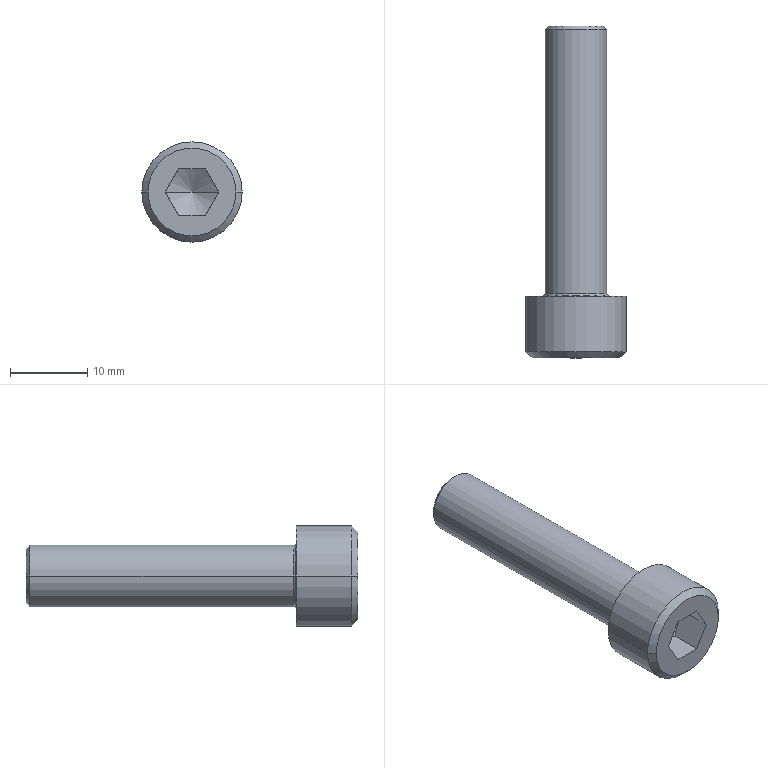Part | Creo | 1 solid | 23 faces | box 13 x 43 x 13 mm | volume 2657 mm3 | plane 9 | cone 6 | cylinder 4 | torus 4 | commonest cylinder face diameters 8 x2 13 x2
STEP:
#1=CARTESIAN_POINT('',(0.,0.,0.));
#2=DIRECTION('',(0.,0.,1.));
#3=DIRECTION('',(1.,0.,0.));
#4=AXIS2_PLACEMENT_3D('',#1,#2,#3);
#5=CARTESIAN_POINT('',(73.036,-244.,-213.));
#6=VERTEX_POINT('',#5);
#7=CARTESIAN_POINT('',(74.768,-244.,-216.));
#8=VERTEX_POINT('',#7);
#9=CARTESIAN_POINT('',(73.036,-244.,-213.));
#10=CARTESIAN_POINT('',(73.087,-243.971,-213.088));
#11=CARTESIAN_POINT('',(73.187,-243.917,-213.261));
#12=CARTESIAN_POINT('',(73.331,-243.851,-213.511));
#13=CARTESIAN_POINT('',(73.473,-243.799,-213.757));
#14=CARTESIAN_POINT('',(73.614,-243.761,-214.002));
#15=CARTESIAN_POINT('',(73.758,-243.737,-214.25));
#16=CARTESIAN_POINT('',(73.902,-243.729,-214.5));
#17=CARTESIAN_POINT('',(74.046,-243.737,-214.75));
#18=CARTESIAN_POINT('',(74.19,-243.761,-214.998));
#19=CARTESIAN_POINT('',(74.331,-243.799,-215.243));
#20=CARTESIAN_POINT('',(74.473,-243.851,-215.489));
#21=CARTESIAN_POINT('',(74.617,-243.917,-215.739));
#22=CARTESIAN_POINT('',(74.717,-243.971,-215.912));
#23=CARTESIAN_POINT('',(74.768,-244.,-216.));
#24=B_SPLINE_CURVE_WITH_KNOTS('',3,(#9,#10,#11,#12,#13,#14,#15,#16,#17,#18,#19,#20,#21,#22,#23),.UNSPECIFIED.,.F.,.F.,(4,1,1,1,1,1,1,1,1,1,1,1,4),(0.,0.08333,0.1667,0.25,0.3333,0.4167,0.5,0.5833,0.6667,0.75,0.8333,0.9167,1.),.UNSPECIFIED.);
#25=EDGE_CURVE('',#6,#8,#24,.T.);
#26=ORIENTED_EDGE('',*,*,#25,.F.);
#27=CARTESIAN_POINT('',(76.5,-242.,-213.));
#28=VERTEX_POINT('',#27);
#29=CARTESIAN_POINT('',(76.5,-242.,-213.));
#30=DIRECTION('',(-0.866,-0.5,0.));
#31=VECTOR('',#30,4.);
#32=LINE('',#29,#31);
#33=EDGE_CURVE('',#28,#6,#32,.T.);
#34=ORIENTED_EDGE('',*,*,#33,.F.);
#35=CARTESIAN_POINT('',(79.964,-244.,-213.));
#36=VERTEX_POINT('',#35);
#37=CARTESIAN_POINT('',(76.5,-242.,-213.));
#38=DIRECTION('',(0.866,-0.5,0.));
#39=VECTOR('',#38,4.);
#40=LINE('',#37,#39);
#41=EDGE_CURVE('',#28,#36,#40,.T.);
#42=ORIENTED_EDGE('',*,*,#41,.T.);
#43=CARTESIAN_POINT('',(78.232,-244.,-216.));
#44=VERTEX_POINT('',#43);
#45=CARTESIAN_POINT('',(78.232,-244.,-216.));
#46=CARTESIAN_POINT('',(78.283,-243.971,-215.912));
#47=CARTESIAN_POINT('',(78.383,-243.917,-215.739));
#48=CARTESIAN_POINT('',(78.527,-243.851,-215.489));
#49=CARTESIAN_POINT('',(78.669,-243.799,-215.243));
#50=CARTESIAN_POINT('',(78.81,-243.761,-214.998));
#51=CARTESIAN_POINT('',(78.954,-243.737,-214.75));
#52=CARTESIAN_POINT('',(79.098,-243.729,-214.5));
#53=CARTESIAN_POINT('',(79.242,-243.737,-214.25));
#54=CARTESIAN_POINT('',(79.386,-243.761,-214.002));
#55=CARTESIAN_POINT('',(79.527,-243.799,-213.757));
#56=CARTESIAN_POINT('',(79.669,-243.851,-213.511));
#57=CARTESIAN_POINT('',(79.813,-243.917,-213.261));
#58=CARTESIAN_POINT('',(79.913,-243.971,-213.088));
#59=CARTESIAN_POINT('',(79.964,-244.,-213.));
#60=B_SPLINE_CURVE_WITH_KNOTS('',3,(#45,#46,#47,#48,#49,#50,#51,#52,#53,#54,#55,#56,#57,#58,#59),.UNSPECIFIED.,.F.,.F.,(4,1,1,1,1,1,1,1,1,1,1,1,4),(0.,0.08333,0.1667,0.25,0.3333,0.4167,0.5,0.5833,0.6667,0.75,0.8333,0.9167,1.),.UNSPECIFIED.);
#61=EDGE_CURVE('',#44,#36,#60,.T.);
#62=ORIENTED_EDGE('',*,*,#61,.F.);
#63=CARTESIAN_POINT('',(74.768,-244.,-216.));
#64=CARTESIAN_POINT('',(74.869,-243.971,-216.));
#65=CARTESIAN_POINT('',(75.069,-243.917,-216.));
#66=CARTESIAN_POINT('',(75.357,-243.851,-216.));
#67=CARTESIAN_POINT('',(75.641,-243.799,-216.));
#68=CARTESIAN_POINT('',(75.924,-243.761,-216.));
#69=CARTESIAN_POINT('',(76.211,-243.737,-216.));
#70=CARTESIAN_POINT('',(76.5,-243.729,-216.));
#71=CARTESIAN_POINT('',(76.789,-243.737,-216.));
#72=CARTESIAN_POINT('',(77.076,-243.761,-216.));
#73=CARTESIAN_POINT('',(77.359,-243.799,-216.));
#74=CARTESIAN_POINT('',(77.643,-243.851,-216.));
#75=CARTESIAN_POINT('',(77.931,-243.917,-216.));
#76=CARTESIAN_POINT('',(78.131,-243.971,-216.));
#77=CARTESIAN_POINT('',(78.232,-244.,-216.));
#78=B_SPLINE_CURVE_WITH_KNOTS('',3,(#63,#64,#65,#66,#67,#68,#69,#70,#71,#72,#73,#74,#75,#76,#77),.UNSPECIFIED.,.F.,.F.,(4,1,1,1,1,1,1,1,1,1,1,1,4),(0.,0.08333,0.1667,0.25,0.3333,0.4167,0.5,0.5833,0.6667,0.75,0.8333,0.9167,1.),.UNSPECIFIED.);
#79=EDGE_CURVE('',#8,#44,#78,.T.);
#80=ORIENTED_EDGE('',*,*,#79,.F.);
#81=EDGE_LOOP('',(#26,#34,#42,#62,#80));
#82=FACE_OUTER_BOUND('',#81,.F.);
#83=CARTESIAN_POINT('',(76.5,-243.02,-213.));
#84=DIRECTION('',(0.,-1.,0.));
#85=DIRECTION('',(-1.,0.,0.));
#86=AXIS2_PLACEMENT_3D('',#83,#84,#85);
#87=CONICAL_SURFACE('',#86,1.767,60.);
#88=ADVANCED_FACE('',(#82),#87,.F.);
#89=CARTESIAN_POINT('',(74.768,-248.,-216.));
#90=VERTEX_POINT('',#89);
#91=CARTESIAN_POINT('',(73.036,-248.,-213.));
#92=VERTEX_POINT('',#91);
#93=CARTESIAN_POINT('',(74.768,-248.,-216.));
#94=DIRECTION('',(-0.5,0.,0.866));
#95=VECTOR('',#94,3.464);
#96=LINE('',#93,#95);
#97=EDGE_CURVE('',#90,#92,#96,.T.);
#98=ORIENTED_EDGE('',*,*,#97,.T.);
#99=CARTESIAN_POINT('',(73.036,-248.,-213.));
#100=DIRECTION('',(0.,1.,0.));
#101=VECTOR('',#100,4.);
#102=LINE('',#99,#101);
#103=EDGE_CURVE('',#92,#6,#102,.T.);
#104=ORIENTED_EDGE('',*,*,#103,.T.);
#105=ORIENTED_EDGE('',*,*,#25,.T.);
#106=CARTESIAN_POINT('',(74.768,-248.,-216.));
#107=DIRECTION('',(0.,1.,0.));
#108=VECTOR('',#107,4.);
#109=LINE('',#106,#108);
#110=EDGE_CURVE('',#90,#8,#109,.T.);
#111=ORIENTED_EDGE('',*,*,#110,.F.);
#112=EDGE_LOOP('',(#98,#104,#105,#111));
#113=FACE_OUTER_BOUND('',#112,.F.);
#114=CARTESIAN_POINT('',(74.768,-244.,-216.));
#115=DIRECTION('',(0.866,0.,0.5));
#116=DIRECTION('',(-0.5,0.,0.866));
#117=AXIS2_PLACEMENT_3D('',#114,#115,#116);
#118=PLANE('',#117);
#119=ADVANCED_FACE('',(#113),#118,.T.);
#120=CARTESIAN_POINT('',(70.8,-248.,-213.));
#121=VERTEX_POINT('',#120);
#122=CARTESIAN_POINT('',(82.2,-248.,-213.));
#123=VERTEX_POINT('',#122);
#124=CARTESIAN_POINT('',(76.5,-248.,-213.));
#125=DIRECTION('',(0.,-1.,0.));
#126=DIRECTION('',(-1.,0.,0.));
#127=AXIS2_PLACEMENT_3D('',#124,#125,#126);
#128=CIRCLE('',#127,5.7);
#129=EDGE_CURVE('',#121,#123,#128,.T.);
#130=ORIENTED_EDGE('',*,*,#129,.F.);
#131=CARTESIAN_POINT('',(76.5,-248.,-213.));
#132=DIRECTION('',(0.,-1.,0.));
#133=DIRECTION('',(1.,0.,0.));
#134=AXIS2_PLACEMENT_3D('',#131,#132,#133);
#135=CIRCLE('',#134,5.7);
#136=EDGE_CURVE('',#123,#121,#135,.T.);
#137=ORIENTED_EDGE('',*,*,#136,.F.);
#138=EDGE_LOOP('',(#130,#137));
#139=FACE_OUTER_BOUND('',#138,.F.);
#140=CARTESIAN_POINT('',(74.768,-248.,-210.));
#141=VERTEX_POINT('',#140);
#142=CARTESIAN_POINT('',(73.036,-248.,-213.));
#143=DIRECTION('',(0.5,0.,0.866));
#144=VECTOR('',#143,3.464);
#145=LINE('',#142,#144);
#146=EDGE_CURVE('',#92,#141,#145,.T.);
#147=ORIENTED_EDGE('',*,*,#146,.F.);
#148=ORIENTED_EDGE('',*,*,#97,.F.);
#149=CARTESIAN_POINT('',(78.232,-248.,-216.));
#150=VERTEX_POINT('',#149);
#151=CARTESIAN_POINT('',(74.768,-248.,-216.));
#152=DIRECTION('',(1.,0.,0.));
#153=VECTOR('',#152,3.464);
#154=LINE('',#151,#153);
#155=EDGE_CURVE('',#90,#150,#154,.T.);
#156=ORIENTED_EDGE('',*,*,#155,.T.);
#157=CARTESIAN_POINT('',(79.964,-248.,-213.));
#158=VERTEX_POINT('',#157);
#159=CARTESIAN_POINT('',(79.964,-248.,-213.));
#160=DIRECTION('',(-0.5,0.,-0.866));
#161=VECTOR('',#160,3.464);
#162=LINE('',#159,#161);
#163=EDGE_CURVE('',#158,#150,#162,.T.);
#164=ORIENTED_EDGE('',*,*,#163,.F.);
#165=CARTESIAN_POINT('',(78.232,-248.,-210.));
#166=VERTEX_POINT('',#165);
#167=CARTESIAN_POINT('',(78.232,-248.,-210.));
#168=DIRECTION('',(0.5,0.,-0.866));
#169=VECTOR('',#168,3.464);
#170=LINE('',#167,#169);
#171=EDGE_CURVE('',#166,#158,#170,.T.);
#172=ORIENTED_EDGE('',*,*,#171,.F.);
#173=CARTESIAN_POINT('',(78.232,-248.,-210.));
#174=DIRECTION('',(-1.,0.,0.));
#175=VECTOR('',#174,3.464);
#176=LINE('',#173,#175);
#177=EDGE_CURVE('',#166,#141,#176,.T.);
#178=ORIENTED_EDGE('',*,*,#177,.T.);
#179=EDGE_LOOP('',(#147,#148,#156,#164,#172,#178));
#180=FACE_BOUND('',#179,.F.);
#181=CARTESIAN_POINT('',(76.5,-248.,-213.));
#182=DIRECTION('',(0.,-1.,0.));
#183=DIRECTION('',(-1.,0.,0.));
#184=AXIS2_PLACEMENT_3D('',#181,#182,#183);
#185=PLANE('',#184);
#186=ADVANCED_FACE('',(#139,#180),#185,.T.);
#187=CARTESIAN_POINT('',(70.,-247.2,-213.));
#188=VERTEX_POINT('',#187);
#189=CARTESIAN_POINT('',(83.,-247.2,-213.));
#190=VERTEX_POINT('',#189);
#191=CARTESIAN_POINT('',(76.5,-247.2,-213.));
#192=DIRECTION('',(0.,-1.,0.));
#193=DIRECTION('',(-1.,0.,0.));
#194=AXIS2_PLACEMENT_3D('',#191,#192,#193);
#195=CIRCLE('',#194,6.5);
#196=EDGE_CURVE('',#188,#190,#195,.T.);
#197=ORIENTED_EDGE('',*,*,#196,.F.);
#198=CARTESIAN_POINT('',(70.8,-248.,-213.));
#199=DIRECTION('',(-0.7071,0.7071,0.));
#200=VECTOR('',#199,1.131);
#201=LINE('',#198,#200);
#202=EDGE_CURVE('',#121,#188,#201,.T.);
#203=ORIENTED_EDGE('',*,*,#202,.F.);
#204=ORIENTED_EDGE('',*,*,#129,.T.);
#205=CARTESIAN_POINT('',(82.2,-248.,-213.));
#206=DIRECTION('',(0.7071,0.7071,0.));
#207=VECTOR('',#206,1.131);
#208=LINE('',#205,#207);
#209=EDGE_CURVE('',#123,#190,#208,.T.);
#210=ORIENTED_EDGE('',*,*,#209,.T.);
#211=EDGE_LOOP('',(#197,#203,#204,#210));
#212=FACE_OUTER_BOUND('',#211,.F.);
#213=CARTESIAN_POINT('',(76.5,-247.6,-213.));
#214=DIRECTION('',(0.,1.,0.));
#215=DIRECTION('',(1.,0.,0.));
#216=AXIS2_PLACEMENT_3D('',#213,#214,#215);
#217=CONICAL_SURFACE('',#216,6.1,45.);
#218=ADVANCED_FACE('',(#212),#217,.T.);
#219=ORIENTED_EDGE('',*,*,#196,.T.);
#220=CARTESIAN_POINT('',(83.,-240.,-213.));
#221=VERTEX_POINT('',#220);
#222=CARTESIAN_POINT('',(83.,-240.,-213.));
#223=DIRECTION('',(0.,-1.,0.));
#224=VECTOR('',#223,7.2);
#225=LINE('',#222,#224);
#226=EDGE_CURVE('',#221,#190,#225,.T.);
#227=ORIENTED_EDGE('',*,*,#226,.F.);
#228=CARTESIAN_POINT('',(70.,-240.,-213.));
#229=VERTEX_POINT('',#228);
#230=CARTESIAN_POINT('',(76.5,-240.,-213.));
#231=DIRECTION('',(0.,1.,0.));
#232=DIRECTION('',(1.,0.,0.));
#233=AXIS2_PLACEMENT_3D('',#230,#231,#232);
#234=CIRCLE('',#233,6.5);
#235=EDGE_CURVE('',#221,#229,#234,.T.);
#236=ORIENTED_EDGE('',*,*,#235,.T.);
#237=CARTESIAN_POINT('',(70.,-240.,-213.));
#238=DIRECTION('',(0.,-1.,0.));
#239=VECTOR('',#238,7.2);
#240=LINE('',#237,#239);
#241=EDGE_CURVE('',#229,#188,#240,.T.);
#242=ORIENTED_EDGE('',*,*,#241,.T.);
#243=EDGE_LOOP('',(#219,#227,#236,#242));
#244=FACE_OUTER_BOUND('',#243,.F.);
#245=CARTESIAN_POINT('',(76.5,-240.,-213.));
#246=DIRECTION('',(0.,-1.,0.));
#247=DIRECTION('',(-1.,0.,0.));
#248=AXIS2_PLACEMENT_3D('',#245,#246,#247);
#249=CYLINDRICAL_SURFACE('',#248,6.5);
#250=ADVANCED_FACE('',(#244),#249,.T.);
#251=CARTESIAN_POINT('',(76.5,-247.2,-213.));
#252=DIRECTION('',(0.,-1.,0.));
#253=DIRECTION('',(1.,0.,0.));
#254=AXIS2_PLACEMENT_3D('',#251,#252,#253);
#255=CIRCLE('',#254,6.5);
#256=EDGE_CURVE('',#190,#188,#255,.T.);
#257=ORIENTED_EDGE('',*,*,#256,.T.);
#258=ORIENTED_EDGE('',*,*,#241,.F.);
#259=CARTESIAN_POINT('',(76.5,-240.,-213.));
#260=DIRECTION('',(0.,1.,0.));
#261=DIRECTION('',(-1.,0.,0.));
#262=AXIS2_PLACEMENT_3D('',#259,#260,#261);
#263=CIRCLE('',#262,6.5);
#264=EDGE_CURVE('',#229,#221,#263,.T.);
#265=ORIENTED_EDGE('',*,*,#264,.T.);
#266=ORIENTED_EDGE('',*,*,#226,.T.);
#267=EDGE_LOOP('',(#257,#258,#265,#266));
#268=FACE_OUTER_BOUND('',#267,.F.);
#269=CARTESIAN_POINT('',(76.5,-240.,-213.));
#270=DIRECTION('',(0.,-1.,0.));
#271=DIRECTION('',(-1.,0.,0.));
#272=AXIS2_PLACEMENT_3D('',#269,#270,#271);
#273=CYLINDRICAL_SURFACE('',#272,6.5);
#274=ADVANCED_FACE('',(#268),#273,.T.);
#275=ORIENTED_EDGE('',*,*,#256,.F.);
#276=ORIENTED_EDGE('',*,*,#209,.F.);
#277=ORIENTED_EDGE('',*,*,#136,.T.);
#278=ORIENTED_EDGE('',*,*,#202,.T.);
#279=EDGE_LOOP('',(#275,#276,#277,#278));
#280=FACE_OUTER_BOUND('',#279,.F.);
#281=CARTESIAN_POINT('',(76.5,-247.6,-213.));
#282=DIRECTION('',(0.,1.,0.));
#283=DIRECTION('',(1.,0.,0.));
#284=AXIS2_PLACEMENT_3D('',#281,#282,#283);
#285=CONICAL_SURFACE('',#284,6.1,45.);
#286=ADVANCED_FACE('',(#280),#285,.T.);
#287=ORIENTED_EDGE('',*,*,#264,.F.);
#288=ORIENTED_EDGE('',*,*,#235,.F.);
#289=EDGE_LOOP('',(#287,#288));
#290=FACE_OUTER_BOUND('',#289,.F.);
#291=CARTESIAN_POINT('',(72.1,-240.,-213.));
#292=VERTEX_POINT('',#291);
#293=CARTESIAN_POINT('',(80.9,-240.,-213.));
#294=VERTEX_POINT('',#293);
#295=CARTESIAN_POINT('',(76.5,-240.,-213.));
#296=DIRECTION('',(0.,-1.,0.));
#297=DIRECTION('',(-1.,0.,0.));
#298=AXIS2_PLACEMENT_3D('',#295,#296,#297);
#299=CIRCLE('',#298,4.4);
#300=EDGE_CURVE('',#292,#294,#299,.T.);
#301=ORIENTED_EDGE('',*,*,#300,.F.);
#302=CARTESIAN_POINT('',(76.5,-240.,-213.));
#303=DIRECTION('',(0.,-1.,0.));
#304=DIRECTION('',(1.,0.,0.));
#305=AXIS2_PLACEMENT_3D('',#302,#303,#304);
#306=CIRCLE('',#305,4.4);
#307=EDGE_CURVE('',#294,#292,#306,.T.);
#308=ORIENTED_EDGE('',*,*,#307,.F.);
#309=EDGE_LOOP('',(#301,#308));
#310=FACE_BOUND('',#309,.F.);
#311=CARTESIAN_POINT('',(76.5,-240.,-213.));
#312=DIRECTION('',(0.,-1.,0.));
#313=DIRECTION('',(-1.,0.,0.));
#314=AXIS2_PLACEMENT_3D('',#311,#312,#313);
#315=PLANE('',#314);
#316=ADVANCED_FACE('',(#290,#310),#315,.F.);
#317=ORIENTED_EDGE('',*,*,#300,.T.);
#318=CARTESIAN_POINT('',(80.617,-239.883,-213.));
#319=VERTEX_POINT('',#318);
#320=CARTESIAN_POINT('',(80.9,-239.6,-213.));
#321=DIRECTION('',(0.,0.,-1.));
#322=DIRECTION('',(0.,-1.,0.));
#323=AXIS2_PLACEMENT_3D('',#320,#321,#322);
#324=CIRCLE('',#323,0.4);
#325=EDGE_CURVE('',#294,#319,#324,.T.);
#326=ORIENTED_EDGE('',*,*,#325,.T.);
#327=CARTESIAN_POINT('',(72.383,-239.883,-213.));
#328=VERTEX_POINT('',#327);
#329=CARTESIAN_POINT('',(76.5,-239.883,-213.));
#330=DIRECTION('',(0.,-1.,0.));
#331=DIRECTION('',(-1.,0.,0.));
#332=AXIS2_PLACEMENT_3D('',#329,#330,#331);
#333=CIRCLE('',#332,4.117);
#334=EDGE_CURVE('',#328,#319,#333,.T.);
#335=ORIENTED_EDGE('',*,*,#334,.F.);
#336=CARTESIAN_POINT('',(72.1,-239.6,-213.));
#337=DIRECTION('',(0.,0.,1.));
#338=DIRECTION('',(0.,-1.,0.));
#339=AXIS2_PLACEMENT_3D('',#336,#337,#338);
#340=CIRCLE('',#339,0.4);
#341=EDGE_CURVE('',#292,#328,#340,.T.);
#342=ORIENTED_EDGE('',*,*,#341,.F.);
#343=EDGE_LOOP('',(#317,#326,#335,#342));
#344=FACE_OUTER_BOUND('',#343,.F.);
#345=CARTESIAN_POINT('',(76.5,-239.6,-213.));
#346=DIRECTION('',(0.,-1.,0.));
#347=DIRECTION('',(-1.,0.,0.));
#348=AXIS2_PLACEMENT_3D('',#345,#346,#347);
#349=TOROIDAL_SURFACE('',#348,4.4,0.4);
#350=ADVANCED_FACE('',(#344),#349,.F.);
#351=ORIENTED_EDGE('',*,*,#307,.T.);
#352=ORIENTED_EDGE('',*,*,#341,.T.);
#353=CARTESIAN_POINT('',(76.5,-239.883,-213.));
#354=DIRECTION('',(0.,-1.,0.));
#355=DIRECTION('',(1.,0.,0.));
#356=AXIS2_PLACEMENT_3D('',#353,#354,#355);
#357=CIRCLE('',#356,4.117);
#358=EDGE_CURVE('',#319,#328,#357,.T.);
#359=ORIENTED_EDGE('',*,*,#358,.F.);
#360=ORIENTED_EDGE('',*,*,#325,.F.);
#361=EDGE_LOOP('',(#351,#352,#359,#360));
#362=FACE_OUTER_BOUND('',#361,.F.);
#363=CARTESIAN_POINT('',(76.5,-239.6,-213.));
#364=DIRECTION('',(0.,-1.,0.));
#365=DIRECTION('',(-1.,0.,0.));
#366=AXIS2_PLACEMENT_3D('',#363,#364,#365);
#367=TOROIDAL_SURFACE('',#366,4.4,0.4);
#368=ADVANCED_FACE('',(#362),#367,.F.);
#369=CARTESIAN_POINT('',(80.5,-239.6,-213.));
#370=VERTEX_POINT('',#369);
#371=CARTESIAN_POINT('',(72.5,-239.6,-213.));
#372=VERTEX_POINT('',#371);
#373=CARTESIAN_POINT('',(76.5,-239.6,-213.));
#374=DIRECTION('',(0.,-1.,0.));
#375=DIRECTION('',(1.,0.,0.));
#376=AXIS2_PLACEMENT_3D('',#373,#374,#375);
#377=CIRCLE('',#376,4.);
#378=EDGE_CURVE('',#370,#372,#377,.T.);
#379=ORIENTED_EDGE('',*,*,#378,.F.);
#380=CARTESIAN_POINT('',(80.9,-239.6,-213.));
#381=DIRECTION('',(0.,0.,-1.));
#382=DIRECTION('',(-0.7071,-0.7071,0.));
#383=AXIS2_PLACEMENT_3D('',#380,#381,#382);
#384=CIRCLE('',#383,0.4);
#385=EDGE_CURVE('',#319,#370,#384,.T.);
#386=ORIENTED_EDGE('',*,*,#385,.F.);
#387=ORIENTED_EDGE('',*,*,#358,.T.);
#388=CARTESIAN_POINT('',(72.1,-239.6,-213.));
#389=DIRECTION('',(0.,0.,1.));
#390=DIRECTION('',(0.7071,-0.7071,0.));
#391=AXIS2_PLACEMENT_3D('',#388,#389,#390);
#392=CIRCLE('',#391,0.4);
#393=EDGE_CURVE('',#328,#372,#392,.T.);
#394=ORIENTED_EDGE('',*,*,#393,.T.);
#395=EDGE_LOOP('',(#379,#386,#387,#394));
#396=FACE_OUTER_BOUND('',#395,.F.);
#397=CARTESIAN_POINT('',(76.5,-239.6,-213.));
#398=DIRECTION('',(0.,-1.,0.));
#399=DIRECTION('',(-1.,0.,0.));
#400=AXIS2_PLACEMENT_3D('',#397,#398,#399);
#401=TOROIDAL_SURFACE('',#400,4.4,0.4);
#402=ADVANCED_FACE('',(#396),#401,.F.);
#403=CARTESIAN_POINT('',(72.5,-205.5,-213.));
#404=VERTEX_POINT('',#403);
#405=CARTESIAN_POINT('',(80.5,-205.5,-213.));
#406=VERTEX_POINT('',#405);
#407=CARTESIAN_POINT('',(76.5,-205.5,-213.));
#408=DIRECTION('',(0.,1.,0.));
#409=DIRECTION('',(-1.,0.,0.));
#410=AXIS2_PLACEMENT_3D('',#407,#408,#409);
#411=CIRCLE('',#410,4.);
#412=EDGE_CURVE('',#404,#406,#411,.T.);
#413=ORIENTED_EDGE('',*,*,#412,.T.);
#414=CARTESIAN_POINT('',(80.5,-205.5,-213.));
#415=DIRECTION('',(0.,-1.,0.));
#416=VECTOR('',#415,34.1);
#417=LINE('',#414,#416);
#418=EDGE_CURVE('',#406,#370,#417,.T.);
#419=ORIENTED_EDGE('',*,*,#418,.T.);
#420=ORIENTED_EDGE('',*,*,#378,.T.);
#421=CARTESIAN_POINT('',(72.5,-205.5,-213.));
#422=DIRECTION('',(0.,-1.,0.));
#423=VECTOR('',#422,34.1);
#424=LINE('',#421,#423);
#425=EDGE_CURVE('',#404,#372,#424,.T.);
#426=ORIENTED_EDGE('',*,*,#425,.F.);
#427=EDGE_LOOP('',(#413,#419,#420,#426));
#428=FACE_OUTER_BOUND('',#427,.F.);
#429=CARTESIAN_POINT('',(76.5,-205.,-213.));
#430=DIRECTION('',(0.,-1.,0.));
#431=DIRECTION('',(-1.,0.,0.));
#432=AXIS2_PLACEMENT_3D('',#429,#430,#431);
#433=CYLINDRICAL_SURFACE('',#432,4.);
#434=ADVANCED_FACE('',(#428),#433,.T.);
#435=CARTESIAN_POINT('',(73.,-205.,-213.));
#436=VERTEX_POINT('',#435);
#437=CARTESIAN_POINT('',(80.,-205.,-213.));
#438=VERTEX_POINT('',#437);
#439=CARTESIAN_POINT('',(76.5,-205.,-213.));
#440=DIRECTION('',(0.,1.,0.));
#441=DIRECTION('',(-1.,0.,0.));
#442=AXIS2_PLACEMENT_3D('',#439,#440,#441);
#443=CIRCLE('',#442,3.5);
#444=EDGE_CURVE('',#436,#438,#443,.T.);
#445=ORIENTED_EDGE('',*,*,#444,.T.);
#446=CARTESIAN_POINT('',(80.,-205.,-213.));
#447=DIRECTION('',(0.7071,-0.7071,0.));
#448=VECTOR('',#447,0.7071);
#449=LINE('',#446,#448);
#450=EDGE_CURVE('',#438,#406,#449,.T.);
#451=ORIENTED_EDGE('',*,*,#450,.T.);
#452=ORIENTED_EDGE('',*,*,#412,.F.);
#453=CARTESIAN_POINT('',(73.,-205.,-213.));
#454=DIRECTION('',(-0.7071,-0.7071,0.));
#455=VECTOR('',#454,0.7071);
#456=LINE('',#453,#455);
#457=EDGE_CURVE('',#436,#404,#456,.T.);
#458=ORIENTED_EDGE('',*,*,#457,.F.);
#459=EDGE_LOOP('',(#445,#451,#452,#458));
#460=FACE_OUTER_BOUND('',#459,.F.);
#461=CARTESIAN_POINT('',(76.5,-205.25,-213.));
#462=DIRECTION('',(0.,-1.,0.));
#463=DIRECTION('',(-1.,0.,0.));
#464=AXIS2_PLACEMENT_3D('',#461,#462,#463);
#465=CONICAL_SURFACE('',#464,3.75,45.);
#466=ADVANCED_FACE('',(#460),#465,.T.);
#467=ORIENTED_EDGE('',*,*,#444,.F.);
#468=CARTESIAN_POINT('',(76.5,-205.,-213.));
#469=DIRECTION('',(0.,1.,0.));
#470=DIRECTION('',(1.,0.,0.));
#471=AXIS2_PLACEMENT_3D('',#468,#469,#470);
#472=CIRCLE('',#471,3.5);
#473=EDGE_CURVE('',#438,#436,#472,.T.);
#474=ORIENTED_EDGE('',*,*,#473,.F.);
#475=EDGE_LOOP('',(#467,#474));
#476=FACE_OUTER_BOUND('',#475,.F.);
#477=CARTESIAN_POINT('',(76.5,-205.,-213.));
#478=DIRECTION('',(0.,-1.,0.));
#479=DIRECTION('',(-1.,0.,0.));
#480=AXIS2_PLACEMENT_3D('',#477,#478,#479);
#481=PLANE('',#480);
#482=ADVANCED_FACE('',(#476),#481,.F.);
#483=ORIENTED_EDGE('',*,*,#473,.T.);
#484=ORIENTED_EDGE('',*,*,#457,.T.);
#485=CARTESIAN_POINT('',(76.5,-205.5,-213.));
#486=DIRECTION('',(0.,1.,0.));
#487=DIRECTION('',(1.,0.,0.));
#488=AXIS2_PLACEMENT_3D('',#485,#486,#487);
#489=CIRCLE('',#488,4.);
#490=EDGE_CURVE('',#406,#404,#489,.T.);
#491=ORIENTED_EDGE('',*,*,#490,.F.);
#492=ORIENTED_EDGE('',*,*,#450,.F.);
#493=EDGE_LOOP('',(#483,#484,#491,#492));
#494=FACE_OUTER_BOUND('',#493,.F.);
#495=CARTESIAN_POINT('',(76.5,-205.25,-213.));
#496=DIRECTION('',(0.,-1.,0.));
#497=DIRECTION('',(-1.,0.,0.));
#498=AXIS2_PLACEMENT_3D('',#495,#496,#497);
#499=CONICAL_SURFACE('',#498,3.75,45.);
#500=ADVANCED_FACE('',(#494),#499,.T.);
#501=ORIENTED_EDGE('',*,*,#490,.T.);
#502=ORIENTED_EDGE('',*,*,#425,.T.);
#503=CARTESIAN_POINT('',(76.5,-239.6,-213.));
#504=DIRECTION('',(0.,-1.,0.));
#505=DIRECTION('',(-1.,0.,0.));
#506=AXIS2_PLACEMENT_3D('',#503,#504,#505);
#507=CIRCLE('',#506,4.);
#508=EDGE_CURVE('',#372,#370,#507,.T.);
#509=ORIENTED_EDGE('',*,*,#508,.T.);
#510=ORIENTED_EDGE('',*,*,#418,.F.);
#511=EDGE_LOOP('',(#501,#502,#509,#510));
#512=FACE_OUTER_BOUND('',#511,.F.);
#513=CARTESIAN_POINT('',(76.5,-205.,-213.));
#514=DIRECTION('',(0.,-1.,0.));
#515=DIRECTION('',(-1.,0.,0.));
#516=AXIS2_PLACEMENT_3D('',#513,#514,#515);
#517=CYLINDRICAL_SURFACE('',#516,4.);
#518=ADVANCED_FACE('',(#512),#517,.T.);
#519=ORIENTED_EDGE('',*,*,#508,.F.);
#520=ORIENTED_EDGE('',*,*,#393,.F.);
#521=ORIENTED_EDGE('',*,*,#334,.T.);
#522=ORIENTED_EDGE('',*,*,#385,.T.);
#523=EDGE_LOOP('',(#519,#520,#521,#522));
#524=FACE_OUTER_BOUND('',#523,.F.);
#525=CARTESIAN_POINT('',(76.5,-239.6,-213.));
#526=DIRECTION('',(0.,-1.,0.));
#527=DIRECTION('',(-1.,0.,0.));
#528=AXIS2_PLACEMENT_3D('',#525,#526,#527);
#529=TOROIDAL_SURFACE('',#528,4.4,0.4);
#530=ADVANCED_FACE('',(#524),#529,.F.);
#531=ORIENTED_EDGE('',*,*,#146,.T.);
#532=CARTESIAN_POINT('',(74.768,-244.,-210.));
#533=VERTEX_POINT('',#532);
#534=CARTESIAN_POINT('',(74.768,-248.,-210.));
#535=DIRECTION('',(0.,1.,0.));
#536=VECTOR('',#535,4.);
#537=LINE('',#534,#536);
#538=EDGE_CURVE('',#141,#533,#537,.T.);
#539=ORIENTED_EDGE('',*,*,#538,.T.);
#540=CARTESIAN_POINT('',(74.768,-244.,-210.));
#541=CARTESIAN_POINT('',(74.717,-243.971,-210.088));
#542=CARTESIAN_POINT('',(74.617,-243.917,-210.261));
#543=CARTESIAN_POINT('',(74.473,-243.851,-210.511));
#544=CARTESIAN_POINT('',(74.331,-243.799,-210.757));
#545=CARTESIAN_POINT('',(74.19,-243.761,-211.002));
#546=CARTESIAN_POINT('',(74.046,-243.737,-211.25));
#547=CARTESIAN_POINT('',(73.902,-243.729,-211.5));
#548=CARTESIAN_POINT('',(73.758,-243.737,-211.75));
#549=CARTESIAN_POINT('',(73.614,-243.761,-211.998));
#550=CARTESIAN_POINT('',(73.473,-243.799,-212.243));
#551=CARTESIAN_POINT('',(73.331,-243.851,-212.489));
#552=CARTESIAN_POINT('',(73.187,-243.917,-212.739));
#553=CARTESIAN_POINT('',(73.087,-243.971,-212.912));
#554=CARTESIAN_POINT('',(73.036,-244.,-213.));
#555=B_SPLINE_CURVE_WITH_KNOTS('',3,(#540,#541,#542,#543,#544,#545,#546,#547,#548,#549,#550,#551,#552,#553,#554),.UNSPECIFIED.,.F.,.F.,(4,1,1,1,1,1,1,1,1,1,1,1,4),(0.,0.08333,0.1667,0.25,0.3333,0.4167,0.5,0.5833,0.6667,0.75,0.8333,0.9167,1.),.UNSPECIFIED.);
#556=EDGE_CURVE('',#533,#6,#555,.T.);
#557=ORIENTED_EDGE('',*,*,#556,.T.);
#558=ORIENTED_EDGE('',*,*,#103,.F.);
#559=EDGE_LOOP('',(#531,#539,#557,#558));
#560=FACE_OUTER_BOUND('',#559,.F.);
#561=CARTESIAN_POINT('',(73.036,-244.,-213.));
#562=DIRECTION('',(0.866,0.,-0.5));
#563=DIRECTION('',(0.5,0.,0.866));
#564=AXIS2_PLACEMENT_3D('',#561,#562,#563);
#565=PLANE('',#564);
#566=ADVANCED_FACE('',(#560),#565,.T.);
#567=ORIENTED_EDGE('',*,*,#177,.F.);
#568=CARTESIAN_POINT('',(78.232,-244.,-210.));
#569=VERTEX_POINT('',#568);
#570=CARTESIAN_POINT('',(78.232,-248.,-210.));
#571=DIRECTION('',(0.,1.,0.));
#572=VECTOR('',#571,4.);
#573=LINE('',#570,#572);
#574=EDGE_CURVE('',#166,#569,#573,.T.);
#575=ORIENTED_EDGE('',*,*,#574,.T.);
#576=CARTESIAN_POINT('',(78.232,-244.,-210.));
#577=CARTESIAN_POINT('',(78.131,-243.971,-210.));
#578=CARTESIAN_POINT('',(77.931,-243.917,-210.));
#579=CARTESIAN_POINT('',(77.643,-243.851,-210.));
#580=CARTESIAN_POINT('',(77.359,-243.799,-210.));
#581=CARTESIAN_POINT('',(77.076,-243.761,-210.));
#582=CARTESIAN_POINT('',(76.789,-243.737,-210.));
#583=CARTESIAN_POINT('',(76.5,-243.729,-210.));
#584=CARTESIAN_POINT('',(76.211,-243.737,-210.));
#585=CARTESIAN_POINT('',(75.924,-243.761,-210.));
#586=CARTESIAN_POINT('',(75.641,-243.799,-210.));
#587=CARTESIAN_POINT('',(75.357,-243.851,-210.));
#588=CARTESIAN_POINT('',(75.069,-243.917,-210.));
#589=CARTESIAN_POINT('',(74.869,-243.971,-210.));
#590=CARTESIAN_POINT('',(74.768,-244.,-210.));
#591=B_SPLINE_CURVE_WITH_KNOTS('',3,(#576,#577,#578,#579,#580,#581,#582,#583,#584,#585,#586,#587,#588,#589,#590),.UNSPECIFIED.,.F.,.F.,(4,1,1,1,1,1,1,1,1,1,1,1,4),(0.,0.08333,0.1667,0.25,0.3333,0.4167,0.5,0.5833,0.6667,0.75,0.8333,0.9167,1.),.UNSPECIFIED.);
#592=EDGE_CURVE('',#569,#533,#591,.T.);
#593=ORIENTED_EDGE('',*,*,#592,.T.);
#594=ORIENTED_EDGE('',*,*,#538,.F.);
#595=EDGE_LOOP('',(#567,#575,#593,#594));
#596=FACE_OUTER_BOUND('',#595,.F.);
#597=CARTESIAN_POINT('',(74.768,-244.,-210.));
#598=DIRECTION('',(0.,0.,-1.));
#599=DIRECTION('',(0.,-1.,0.));
#600=AXIS2_PLACEMENT_3D('',#597,#598,#599);
#601=PLANE('',#600);
#602=ADVANCED_FACE('',(#596),#601,.T.);
#603=ORIENTED_EDGE('',*,*,#171,.T.);
#604=CARTESIAN_POINT('',(79.964,-248.,-213.));
#605=DIRECTION('',(0.,1.,0.));
#606=VECTOR('',#605,4.);
#607=LINE('',#604,#606);
#608=EDGE_CURVE('',#158,#36,#607,.T.);
#609=ORIENTED_EDGE('',*,*,#608,.T.);
#610=CARTESIAN_POINT('',(79.964,-244.,-213.));
#611=CARTESIAN_POINT('',(79.913,-243.971,-212.912));
#612=CARTESIAN_POINT('',(79.813,-243.917,-212.739));
#613=CARTESIAN_POINT('',(79.669,-243.851,-212.489));
#614=CARTESIAN_POINT('',(79.527,-243.799,-212.243));
#615=CARTESIAN_POINT('',(79.386,-243.761,-211.998));
#616=CARTESIAN_POINT('',(79.242,-243.737,-211.75));
#617=CARTESIAN_POINT('',(79.098,-243.729,-211.5));
#618=CARTESIAN_POINT('',(78.954,-243.737,-211.25));
#619=CARTESIAN_POINT('',(78.81,-243.761,-211.002));
#620=CARTESIAN_POINT('',(78.669,-243.799,-210.757));
#621=CARTESIAN_POINT('',(78.527,-243.851,-210.511));
#622=CARTESIAN_POINT('',(78.383,-243.917,-210.261));
#623=CARTESIAN_POINT('',(78.283,-243.971,-210.088));
#624=CARTESIAN_POINT('',(78.232,-244.,-210.));
#625=B_SPLINE_CURVE_WITH_KNOTS('',3,(#610,#611,#612,#613,#614,#615,#616,#617,#618,#619,#620,#621,#622,#623,#624),.UNSPECIFIED.,.F.,.F.,(4,1,1,1,1,1,1,1,1,1,1,1,4),(0.,0.08333,0.1667,0.25,0.3333,0.4167,0.5,0.5833,0.6667,0.75,0.8333,0.9167,1.),.UNSPECIFIED.);
#626=EDGE_CURVE('',#36,#569,#625,.T.);
#627=ORIENTED_EDGE('',*,*,#626,.T.);
#628=ORIENTED_EDGE('',*,*,#574,.F.);
#629=EDGE_LOOP('',(#603,#609,#627,#628));
#630=FACE_OUTER_BOUND('',#629,.F.);
#631=CARTESIAN_POINT('',(78.232,-244.,-210.));
#632=DIRECTION('',(-0.866,0.,-0.5));
#633=DIRECTION('',(0.5,0.,-0.866));
#634=AXIS2_PLACEMENT_3D('',#631,#632,#633);
#635=PLANE('',#634);
#636=ADVANCED_FACE('',(#630),#635,.T.);
#637=ORIENTED_EDGE('',*,*,#163,.T.);
#638=CARTESIAN_POINT('',(78.232,-248.,-216.));
#639=DIRECTION('',(0.,1.,0.));
#640=VECTOR('',#639,4.);
#641=LINE('',#638,#640);
#642=EDGE_CURVE('',#150,#44,#641,.T.);
#643=ORIENTED_EDGE('',*,*,#642,.T.);
#644=ORIENTED_EDGE('',*,*,#61,.T.);
#645=ORIENTED_EDGE('',*,*,#608,.F.);
#646=EDGE_LOOP('',(#637,#643,#644,#645));
#647=FACE_OUTER_BOUND('',#646,.F.);
#648=CARTESIAN_POINT('',(79.964,-244.,-213.));
#649=DIRECTION('',(-0.866,0.,0.5));
#650=DIRECTION('',(-0.5,0.,-0.866));
#651=AXIS2_PLACEMENT_3D('',#648,#649,#650);
#652=PLANE('',#651);
#653=ADVANCED_FACE('',(#647),#652,.T.);
#654=ORIENTED_EDGE('',*,*,#155,.F.);
#655=ORIENTED_EDGE('',*,*,#110,.T.);
#656=ORIENTED_EDGE('',*,*,#79,.T.);
#657=ORIENTED_EDGE('',*,*,#642,.F.);
#658=EDGE_LOOP('',(#654,#655,#656,#657));
#659=FACE_OUTER_BOUND('',#658,.F.);
#660=CARTESIAN_POINT('',(78.232,-244.,-216.));
#661=DIRECTION('',(0.,0.,1.));
#662=DIRECTION('',(0.,1.,0.));
#663=AXIS2_PLACEMENT_3D('',#660,#661,#662);
#664=PLANE('',#663);
#665=ADVANCED_FACE('',(#659),#664,.T.);
#666=ORIENTED_EDGE('',*,*,#626,.F.);
#667=ORIENTED_EDGE('',*,*,#41,.F.);
#668=ORIENTED_EDGE('',*,*,#33,.T.);
#669=ORIENTED_EDGE('',*,*,#556,.F.);
#670=ORIENTED_EDGE('',*,*,#592,.F.);
#671=EDGE_LOOP('',(#666,#667,#668,#669,#670));
#672=FACE_OUTER_BOUND('',#671,.F.);
#673=CARTESIAN_POINT('',(76.5,-243.02,-213.));
#674=DIRECTION('',(0.,-1.,0.));
#675=DIRECTION('',(-1.,0.,0.));
#676=AXIS2_PLACEMENT_3D('',#673,#674,#675);
#677=CONICAL_SURFACE('',#676,1.767,60.);
#678=ADVANCED_FACE('',(#672),#677,.F.);
#679=CLOSED_SHELL('',(#88,#119,#186,#218,#250,#274,#286,#316,#350,#368,#402,#434,#466,#482,#500,#518,#530,#566,#602,#636,#653,#665,#678));
#680=MANIFOLD_SOLID_BREP('',#679);
#681=(LENGTH_UNIT()NAMED_UNIT(*)SI_UNIT(.MILLI.,.METRE.));
#682=UNCERTAINTY_MEASURE_WITH_UNIT(LENGTH_MEASURE(0.004677),#681,'','');
#683=(NAMED_UNIT(*)PLANE_ANGLE_UNIT()SI_UNIT($,.RADIAN.));
#684=PLANE_ANGLE_MEASURE_WITH_UNIT(PLANE_ANGLE_MEASURE(0.01745),#683);
#685=(CONVERSION_BASED_UNIT('DEGREE',#684)NAMED_UNIT(*)PLANE_ANGLE_UNIT());
#686=(NAMED_UNIT(*)SI_UNIT($,.STERADIAN.)SOLID_ANGLE_UNIT());
#687=(GEOMETRIC_REPRESENTATION_CONTEXT(3)GLOBAL_UNCERTAINTY_ASSIGNED_CONTEXT((#682))GLOBAL_UNIT_ASSIGNED_CONTEXT((#681,#685,#686))REPRESENTATION_CONTEXT('',''));
#688=ADVANCED_BREP_SHAPE_REPRESENTATION('',(#4,#680),#687);